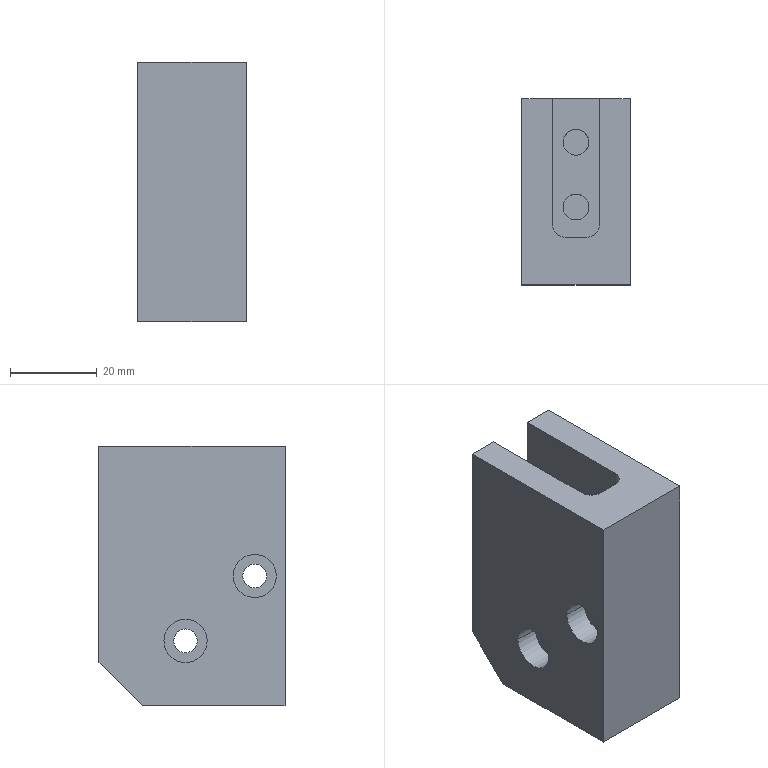Part | SolidWorks | features ICE 9, HoleWzd 3, Chamfer 1, Cut 1, ExtruThin 1, Fillet 1 | 1 solid | 45 faces | box 25 x 43 x 60 mm | volume 52807 mm3 | cylinder 26 | plane 17 | cone 2 | commonest cylinder face diameters 10 x8 6 x6 2.5 x4 4.2 x4 5.5 x4